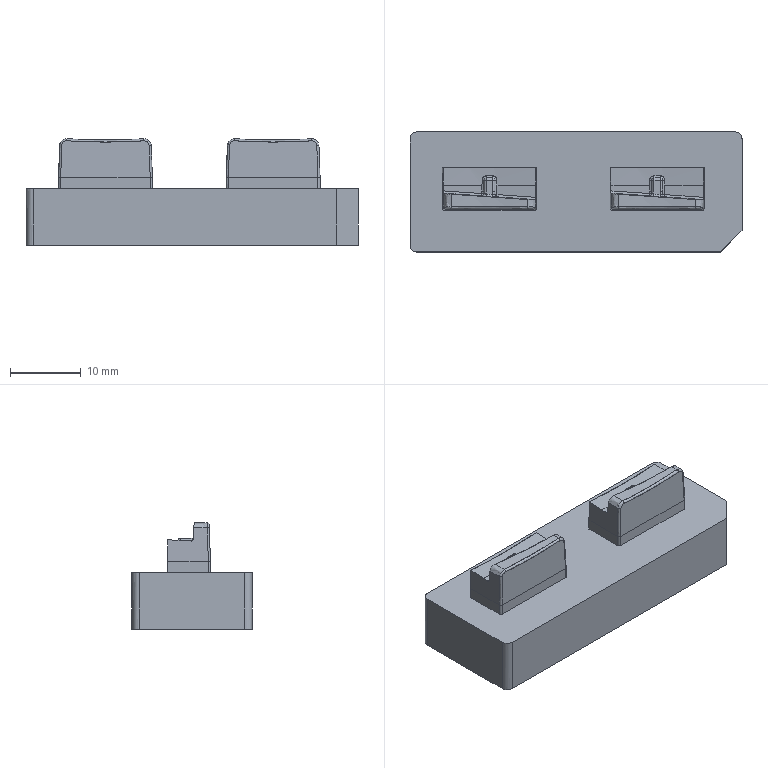CAM job | PowerMill | 3-axis milling, other | part box 47 x 17 x 15.061 mm
Tools:
number,name,type,diameter,tip_radius,length,cutting_length,overhang,flutes,holder,toolpaths_using
1,D10C,end_mill,10.0,0.0,60.0,,30.0,1,D42L35,2
2,D4C,end_mill,4.0,0.0,30.0,,15.0,1,D42L35,2
1,D10C_1_1,end_mill,10.0,0.0,60.0,,15.52,1,D42L35,6
2,D4C_1_1,end_mill,4.0,0.0,30.0,,7.24,1,D42L35,2
27,D1C_1_1,end_mill,1.0,0.0,3.0,,3.04,1,D42L35,2
3,D10_1_1,end_mill,10.0,0.0,60.0,,15.24,1,D42L35,6
4,R1_1_1,ball_nosed,2.0,1.0,6.52,,6.84,1,D42L35,1
6,R0.5_1_1,ball_nosed,1.0,0.5,3.0,,3.16,1,D42L35,1
25,R0.3_1_1,ball_nosed,0.6,0.3,3.0,,3.08,1,D42L35,2
13,Text_D4_1_1,taper_spherical,4.0,0.3,60.0,,7.32,1,D42L35,2
2,D4C_2_1,end_mill,4.0,0.0,30.0,,7.12,1,D42L35,2
4,R1_2_1,ball_nosed,2.0,1.0,6.48,,6.68,1,D42L35,1
6,R0.5_2_1,ball_nosed,1.0,0.5,3.0,,3.12,1,D42L35,1
Operations:
program,toolpath,strategy,tool,tool_number,tool_diameter,tip_radius,flutes,spindle_rpm,feed_cut,surface_speed_m_min_computed,feed_per_tooth_computed,tolerance,thickness,stepover,stepdown,cut_length,cut_time_min,total_time_min,workplane
20-D01-4-F,精公开粗01-扫面平行-D10C,raster_area_clear,D10C_1_1,1,10.0,0.0,1.0,8000.0,10000.0,251.33,1.25,0.03,0.28,6.0,1.0,285.36,0.029,0.035,
20-D01-4-F,精公开粗01-外形偏置-D10C,offset_area_clear,D10C_1_1,1,10.0,0.0,1.0,8000.0,10000.0,251.33,1.25,0.03,0.28,6.0,1.0,5103.558,0.51,0.5578,
20-D01-4-F,精公开粗01-基准台等高-D10C,constantz,D10C_1_1,1,10.0,0.0,1.0,8000.0,10000.0,251.33,1.25,0.03,0.07,5.0,0.4,3449.033,0.345,0.3542,
20-D01-4-F,精公再粗02-外形偏置-D4C,offset_area_clear,D4C_1_1,2,4.0,0.0,1.0,18000.0,6000.0,226.19,0.3333,0.03,0.0,2.0,1.0,3990.108,0.665,0.7406,
20-D01-4-F,精公再粗02-平行中光-D4C,raster,D4C_1_1,2,4.0,0.0,1.0,18000.0,6000.0,226.19,0.3333,0.03,0.0,0.2,1.0,1485.387,0.248,0.2731,
20-D01-4-F,精公再粗03-外形偏置-D1C,offset_area_clear,D1C_1_1,27,1.0,0.0,1.0,22000.0,2000.0,69.12,0.0909,0.03,0.0,0.5,1.0,212.759,0.106,0.2808,
20-D01-4-F,精公基准台01-基准面偏置-D10,offset_area_clear,D10_1_1,3,10.0,0.0,1.0,8500.0,600.0,267.04,0.0706,0.005,0.38,5.0,1.0,132.297,0.221,0.2379,
20-D01-4-F,精公基准台01-外形侧光-D10,profile_area_clear,D10_1_1,3,10.0,0.0,1.0,8500.0,600.0,267.04,0.0706,0.005,-0.07,0.08,1.0,278.722,0.465,0.5027,
20-D01-4-F,精公基准台01-基准台侧光-D10,profile_area_clear,D10_1_1,3,10.0,0.0,1.0,8500.0,600.0,267.04,0.0706,0.005,0.0,0.08,1.0,313.233,0.522,0.586,
20-D01-4-F,精公精光01-浅滩和陡峭-R1,inter_constz,R1_1_1,4,2.0,1.0,1.0,18000.0,2000.0,113.1,0.1111,0.005,-0.075,0.03,1.0,18838.059,9.419,9.889,
20-D01-4-F,精公精光02-清角-R0.5,automatic_corner,R0.5_1_1,6,1.0,0.5,1.0,20000.0,1000.0,62.83,0.05,0.005,-0.075,5.0,1.0,3513.1,3.513,3.678,
20-D01-4-F,精公精光03-清角-R0.3,automatic_corner,R0.3_1_1,25,0.6,0.3,1.0,23000.0,1000.0,43.35,0.0435,0.005,-0.075,5.0,1.0,3426.806,3.427,3.55,
20-D01-4-F,精公刻字01-刻字-Text_D4,pattern,Text_D4_1_1,13,4.0,0.3,1.0,15000.0,1000.0,188.5,0.0667,0.005,0.0,5.0,1.0,71.656,0.072,0.0906,
20-D01-4-R,粗公开粗01-扫面平行-D10C,raster_area_clear,D10C_1_1,1,10.0,0.0,1.0,8000.0,10000.0,251.33,1.25,0.03,0.15,6.0,1.0,283.8,0.028,0.0348,
20-D01-4-R,粗公开粗01-外形偏置-D10C,offset_area_clear,D10C_1_1,1,10.0,0.0,1.0,8000.0,10000.0,251.33,1.25,0.03,0.15,6.0,1.0,5212.288,0.521,0.5688,
20-D01-4-R,粗公开粗01-基准台等高-D10C,constantz,D10C_1_1,1,10.0,0.0,1.0,8000.0,10000.0,251.33,1.25,0.03,0.07,5.0,0.4,3449.033,0.345,0.3542,
20-D01-4-R,粗公再粗02-外形偏置-D4C,offset_area_clear,D4C_2_1,2,4.0,0.0,1.0,18000.0,6000.0,226.19,0.3333,0.03,-0.13,2.0,1.0,3391.719,0.565,0.5953,
20-D01-4-R,粗公再粗02-平行中光-D4C,raster,D4C_2_1,2,4.0,0.0,1.0,18000.0,6000.0,226.19,0.3333,0.03,-0.13,0.2,1.0,1416.638,0.236,0.2617,
20-D01-4-R,粗公再粗03-外形偏置-D1C,offset_area_clear,D1C_1_1,27,1.0,0.0,1.0,22000.0,2000.0,69.12,0.0909,0.03,-0.13,0.5,1.0,221.394,0.111,0.2963,
20-D01-4-R,粗公基准台01-基准面偏置-D10,offset_area_clear,D10_1_1,3,10.0,0.0,1.0,8500.0,600.0,267.04,0.0706,0.01,0.25,5.0,1.0,133.216,0.222,0.2409,
20-D01-4-R,粗公基准台01-外形侧光-D10,profile_area_clear,D10_1_1,3,10.0,0.0,1.0,8500.0,600.0,267.04,0.0706,0.01,-0.2,0.08,1.0,275.442,0.459,0.4972,
20-D01-4-R,粗公基准台01-基准台侧光-D10,profile_area_clear,D10_1_1,3,10.0,0.0,1.0,8500.0,600.0,267.04,0.0706,0.01,0.0,0.08,1.0,313.216,0.522,0.5859,
20-D01-4-R,粗公精光01-浅滩和陡峭-R1,inter_constz,R1_2_1,4,2.0,1.0,1.0,18000.0,2000.0,113.1,0.1111,0.01,-0.205,0.036,1.0,15281.33,7.641,8.049,
20-D01-4-R,粗公精光02-清角-R0.5,automatic_corner,R0.5_2_1,6,1.0,0.5,1.0,20000.0,1000.0,62.83,0.05,0.01,-0.205,5.0,1.0,2754.992,2.755,2.902,
20-D01-4-R,粗公精光03-清角-R0.3,automatic_corner,R0.3_1_1,25,0.6,0.3,1.0,23000.0,1000.0,43.35,0.0435,0.01,-0.205,5.0,1.0,2633.095,2.633,2.739,
20-D01-4-R,粗公刻字01-刻字-Text_D4,pattern,Text_D4_1_1,13,4.0,0.3,1.0,15000.0,1000.0,188.5,0.0667,0.01,0.0,5.0,1.0,69.38,0.069,0.0874,
,精公开粗01-外形偏置-D10C_Reference,offset_area_clear,D10C,1,10.0,0.0,1.0,8000.0,10000.0,251.33,1.25,0.03,0.28,6.0,1.0,9923.648,0.992,1.081,
,精公再粗02-外形偏置-D4C_Reference,offset_area_clear,D4C,2,4.0,0.0,1.0,18000.0,6000.0,226.19,0.3333,0.03,0.0,2.0,1.0,14894.954,2.482,2.773,
,粗公开粗01-外形偏置-D10C_Reference,offset_area_clear,D10C,1,10.0,0.0,1.0,8000.0,10000.0,251.33,1.25,0.03,0.15,6.0,1.0,10131.445,1.013,1.102,
,粗公再粗02-外形偏置-D4C_Reference,offset_area_clear,D4C,2,4.0,0.0,1.0,18000.0,6000.0,226.19,0.3333,0.03,-0.13,2.0,1.0,13463.861,2.244,2.367,